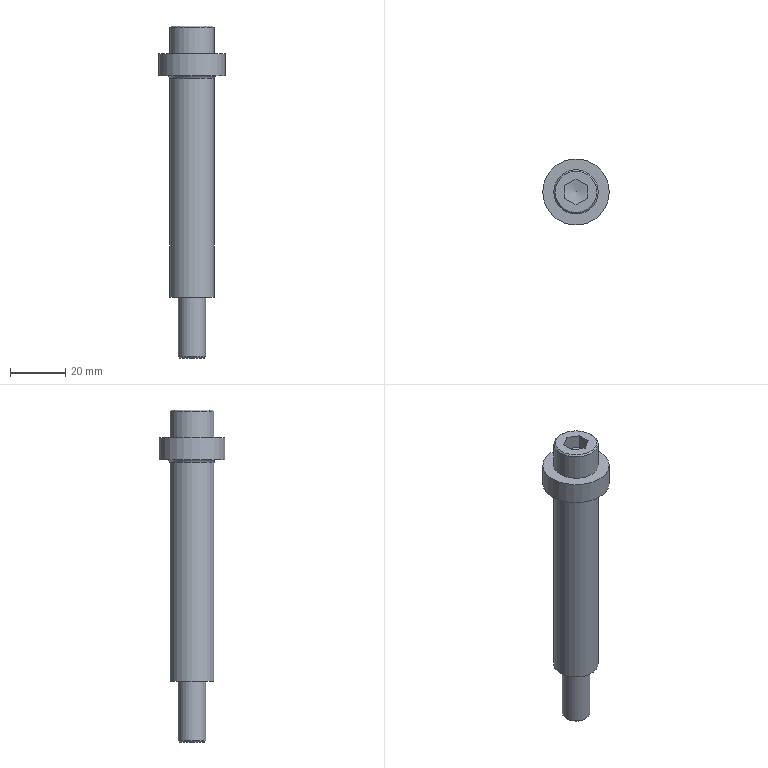Part | NX | features CSR16-70_1 2 | 1 solid | 27 faces | box 24 x 24 x 120 mm | volume 22290 mm3 | plane 18 | cylinder 5 | cone 3 | torus 1 | commonest cylinder face diameters 16 x2 10 x1 10.6 x1 24 x1
STEP:
#1=CARTESIAN_POINT('',(254.,112.,128.));
#2=VERTEX_POINT('',#1);
#3=CARTESIAN_POINT('',(266.,112.,128.));
#4=DIRECTION('',(0.,0.,-1.));
#5=DIRECTION('',(-1.,0.,0.));
#6=AXIS2_PLACEMENT_3D('',#3,#4,#5);
#7=CIRCLE('',#6,12.);
#8=EDGE_CURVE('',#2,#2,#7,.F.);
#9=ORIENTED_EDGE('',*,*,#8,.T.);
#10=EDGE_LOOP('',(#9));
#11=FACE_BOUND('',#10,.T.);
#12=CARTESIAN_POINT('',(258.,112.,128.));
#13=VERTEX_POINT('',#12);
#14=CARTESIAN_POINT('',(266.,112.,128.));
#15=DIRECTION('',(0.,0.,1.));
#16=DIRECTION('',(-1.,0.,0.));
#17=AXIS2_PLACEMENT_3D('',#14,#15,#16);
#18=CIRCLE('',#17,8.);
#19=EDGE_CURVE('',#13,#13,#18,.F.);
#20=ORIENTED_EDGE('',*,*,#19,.T.);
#21=EDGE_LOOP('',(#20));
#22=FACE_BOUND('',#21,.T.);
#23=CARTESIAN_POINT('',(266.,112.,128.));
#24=DIRECTION('',(0.,0.,1.));
#25=DIRECTION('',(-1.,0.,0.));
#26=AXIS2_PLACEMENT_3D('',#23,#24,#25);
#27=PLANE('',#26);
#28=ADVANCED_FACE('',(#11,#22),#27,.T.);
#29=CARTESIAN_POINT('',(258.,112.,119.));
#30=VERTEX_POINT('',#29);
#31=CARTESIAN_POINT('',(266.,112.,119.));
#32=DIRECTION('',(0.,0.,-1.));
#33=DIRECTION('',(1.,0.,0.));
#34=AXIS2_PLACEMENT_3D('',#31,#32,#33);
#35=CIRCLE('',#34,8.);
#36=EDGE_CURVE('',#30,#30,#35,.F.);
#37=ORIENTED_EDGE('',*,*,#36,.F.);
#38=EDGE_LOOP('',(#37));
#39=FACE_BOUND('',#38,.T.);
#40=CARTESIAN_POINT('',(258.,112.,40.));
#41=VERTEX_POINT('',#40);
#42=CARTESIAN_POINT('',(266.,112.,40.));
#43=DIRECTION('',(0.,0.,1.));
#44=DIRECTION('',(-1.,0.,0.));
#45=AXIS2_PLACEMENT_3D('',#42,#43,#44);
#46=CIRCLE('',#45,8.);
#47=EDGE_CURVE('',#41,#41,#46,.F.);
#48=ORIENTED_EDGE('',*,*,#47,.F.);
#49=EDGE_LOOP('',(#48));
#50=FACE_BOUND('',#49,.T.);
#51=CARTESIAN_POINT('',(266.,112.,75.));
#52=DIRECTION('',(0.,0.,-1.));
#53=DIRECTION('',(1.,0.,0.));
#54=AXIS2_PLACEMENT_3D('',#51,#52,#53);
#55=CYLINDRICAL_SURFACE('',#54,8.);
#56=ADVANCED_FACE('',(#39,#50),#55,.T.);
#57=CARTESIAN_POINT('',(260.7,112.,128.));
#58=VERTEX_POINT('',#57);
#59=CARTESIAN_POINT('',(266.,112.,128.));
#60=DIRECTION('',(0.,0.,1.));
#61=DIRECTION('',(-1.,0.,0.));
#62=AXIS2_PLACEMENT_3D('',#59,#60,#61);
#63=CIRCLE('',#62,5.3);
#64=EDGE_CURVE('',#58,#58,#63,.F.);
#65=ORIENTED_EDGE('',*,*,#64,.F.);
#66=EDGE_LOOP('',(#65));
#67=FACE_BOUND('',#66,.T.);
#68=CARTESIAN_POINT('',(260.7,112.,40.));
#69=VERTEX_POINT('',#68);
#70=CARTESIAN_POINT('',(266.,112.,40.));
#71=DIRECTION('',(0.,0.,-1.));
#72=DIRECTION('',(-1.,0.,0.));
#73=AXIS2_PLACEMENT_3D('',#70,#71,#72);
#74=CIRCLE('',#73,5.3);
#75=EDGE_CURVE('',#69,#69,#74,.F.);
#76=ORIENTED_EDGE('',*,*,#75,.F.);
#77=EDGE_LOOP('',(#76));
#78=FACE_BOUND('',#77,.T.);
#79=CARTESIAN_POINT('',(266.,112.,79.));
#80=DIRECTION('',(0.,0.,-1.));
#81=DIRECTION('',(1.,0.,0.));
#82=AXIS2_PLACEMENT_3D('',#79,#80,#81);
#83=CYLINDRICAL_SURFACE('',#82,5.3);
#84=ADVANCED_FACE('',(#67,#78),#83,.F.);
#85=ORIENTED_EDGE('',*,*,#36,.T.);
#86=EDGE_LOOP('',(#85));
#87=FACE_BOUND('',#86,.T.);
#88=CARTESIAN_POINT('',(257.,112.,120.));
#89=VERTEX_POINT('',#88);
#90=CARTESIAN_POINT('',(266.,112.,120.));
#91=DIRECTION('',(0.,0.,1.));
#92=DIRECTION('',(1.,0.,0.));
#93=AXIS2_PLACEMENT_3D('',#90,#91,#92);
#94=CIRCLE('',#93,9.);
#95=EDGE_CURVE('',#89,#89,#94,.F.);
#96=ORIENTED_EDGE('',*,*,#95,.T.);
#97=EDGE_LOOP('',(#96));
#98=FACE_BOUND('',#97,.T.);
#99=CARTESIAN_POINT('',(266.,112.,119.));
#100=DIRECTION('',(0.,0.,1.));
#101=DIRECTION('',(-1.,0.,0.));
#102=AXIS2_PLACEMENT_3D('',#99,#100,#101);
#103=TOROIDAL_SURFACE('',#102,9.,1.);
#104=ADVANCED_FACE('',(#87,#98),#103,.F.);
#105=CARTESIAN_POINT('',(254.,112.,120.));
#106=VERTEX_POINT('',#105);
#107=CARTESIAN_POINT('',(266.,112.,120.));
#108=DIRECTION('',(0.,0.,1.));
#109=DIRECTION('',(-1.,0.,0.));
#110=AXIS2_PLACEMENT_3D('',#107,#108,#109);
#111=CIRCLE('',#110,12.);
#112=EDGE_CURVE('',#106,#106,#111,.F.);
#113=ORIENTED_EDGE('',*,*,#112,.T.);
#114=EDGE_LOOP('',(#113));
#115=FACE_BOUND('',#114,.T.);
#116=ORIENTED_EDGE('',*,*,#95,.F.);
#117=EDGE_LOOP('',(#116));
#118=FACE_BOUND('',#117,.T.);
#119=CARTESIAN_POINT('',(266.,112.,120.));
#120=DIRECTION('',(0.,0.,-1.));
#121=DIRECTION('',(1.,0.,0.));
#122=AXIS2_PLACEMENT_3D('',#119,#120,#121);
#123=PLANE('',#122);
#124=ADVANCED_FACE('',(#115,#118),#123,.T.);
#125=ORIENTED_EDGE('',*,*,#75,.T.);
#126=EDGE_LOOP('',(#125));
#127=FACE_BOUND('',#126,.T.);
#128=ORIENTED_EDGE('',*,*,#47,.T.);
#129=EDGE_LOOP('',(#128));
#130=FACE_BOUND('',#129,.T.);
#131=CARTESIAN_POINT('',(266.,112.,40.));
#132=DIRECTION('',(0.,0.,-1.));
#133=DIRECTION('',(1.,0.,0.));
#134=AXIS2_PLACEMENT_3D('',#131,#132,#133);
#135=PLANE('',#134);
#136=ADVANCED_FACE('',(#127,#130),#135,.T.);
#137=ORIENTED_EDGE('',*,*,#8,.F.);
#138=EDGE_LOOP('',(#137));
#139=FACE_BOUND('',#138,.T.);
#140=ORIENTED_EDGE('',*,*,#112,.F.);
#141=EDGE_LOOP('',(#140));
#142=FACE_BOUND('',#141,.T.);
#143=CARTESIAN_POINT('',(266.,112.,124.));
#144=DIRECTION('',(0.,0.,-1.));
#145=DIRECTION('',(1.,0.,0.));
#146=AXIS2_PLACEMENT_3D('',#143,#144,#145);
#147=CYLINDRICAL_SURFACE('',#146,12.);
#148=ADVANCED_FACE('',(#139,#142),#147,.T.);
#149=CARTESIAN_POINT('',(262.,114.309,138.));
#150=VERTEX_POINT('',#149);
#151=CARTESIAN_POINT('',(266.,116.619,138.));
#152=VERTEX_POINT('',#151);
#153=CARTESIAN_POINT('',(264.,115.464,138.));
#154=DIRECTION('',(-0.866,-0.5,0.));
#155=VECTOR('',#154,1000.);
#156=LINE('',#153,#155);
#157=EDGE_CURVE('',#150,#152,#156,.F.);
#158=ORIENTED_EDGE('',*,*,#157,.T.);
#159=CARTESIAN_POINT('',(270.,114.309,138.));
#160=VERTEX_POINT('',#159);
#161=CARTESIAN_POINT('',(268.,115.464,138.));
#162=DIRECTION('',(-0.866,0.5,0.));
#163=VECTOR('',#162,1000.);
#164=LINE('',#161,#163);
#165=EDGE_CURVE('',#152,#160,#164,.F.);
#166=ORIENTED_EDGE('',*,*,#165,.T.);
#167=CARTESIAN_POINT('',(270.,109.691,138.));
#168=VERTEX_POINT('',#167);
#169=CARTESIAN_POINT('',(270.,112.,138.));
#170=DIRECTION('',(0.,1.,0.));
#171=VECTOR('',#170,1000.);
#172=LINE('',#169,#171);
#173=EDGE_CURVE('',#160,#168,#172,.F.);
#174=ORIENTED_EDGE('',*,*,#173,.T.);
#175=CARTESIAN_POINT('',(266.,107.381,138.));
#176=VERTEX_POINT('',#175);
#177=CARTESIAN_POINT('',(268.,108.536,138.));
#178=DIRECTION('',(0.866,0.5,0.));
#179=VECTOR('',#178,1000.);
#180=LINE('',#177,#179);
#181=EDGE_CURVE('',#168,#176,#180,.F.);
#182=ORIENTED_EDGE('',*,*,#181,.T.);
#183=CARTESIAN_POINT('',(262.,109.691,138.));
#184=VERTEX_POINT('',#183);
#185=CARTESIAN_POINT('',(264.,108.536,138.));
#186=DIRECTION('',(0.866,-0.5,0.));
#187=VECTOR('',#186,1000.);
#188=LINE('',#185,#187);
#189=EDGE_CURVE('',#176,#184,#188,.F.);
#190=ORIENTED_EDGE('',*,*,#189,.T.);
#191=CARTESIAN_POINT('',(262.,112.,138.));
#192=DIRECTION('',(0.,-1.,0.));
#193=VECTOR('',#192,1000.);
#194=LINE('',#191,#193);
#195=EDGE_CURVE('',#184,#150,#194,.F.);
#196=ORIENTED_EDGE('',*,*,#195,.T.);
#197=EDGE_LOOP('',(#158,#166,#174,#182,#190,#196));
#198=FACE_BOUND('',#197,.T.);
#199=CARTESIAN_POINT('',(258.5,112.,138.));
#200=VERTEX_POINT('',#199);
#201=CARTESIAN_POINT('',(266.,112.,138.));
#202=DIRECTION('',(0.,0.,1.));
#203=DIRECTION('',(1.,0.,0.));
#204=AXIS2_PLACEMENT_3D('',#201,#202,#203);
#205=CIRCLE('',#204,7.5);
#206=EDGE_CURVE('',#200,#200,#205,.F.);
#207=ORIENTED_EDGE('',*,*,#206,.F.);
#208=EDGE_LOOP('',(#207));
#209=FACE_BOUND('',#208,.T.);
#210=CARTESIAN_POINT('',(266.,112.,138.));
#211=DIRECTION('',(0.,0.,1.));
#212=DIRECTION('',(-1.,0.,0.));
#213=AXIS2_PLACEMENT_3D('',#210,#211,#212);
#214=PLANE('',#213);
#215=ADVANCED_FACE('',(#198,#209),#214,.T.);
#216=ORIENTED_EDGE('',*,*,#19,.F.);
#217=EDGE_LOOP('',(#216));
#218=FACE_BOUND('',#217,.T.);
#219=CARTESIAN_POINT('',(258.,112.,137.5));
#220=VERTEX_POINT('',#219);
#221=CARTESIAN_POINT('',(266.,112.,137.5));
#222=DIRECTION('',(0.,0.,-1.));
#223=DIRECTION('',(1.,0.,0.));
#224=AXIS2_PLACEMENT_3D('',#221,#222,#223);
#225=CIRCLE('',#224,8.);
#226=EDGE_CURVE('',#220,#220,#225,.F.);
#227=ORIENTED_EDGE('',*,*,#226,.F.);
#228=EDGE_LOOP('',(#227));
#229=FACE_BOUND('',#228,.T.);
#230=CARTESIAN_POINT('',(266.,112.,133.));
#231=DIRECTION('',(0.,0.,-1.));
#232=DIRECTION('',(1.,0.,0.));
#233=AXIS2_PLACEMENT_3D('',#230,#231,#232);
#234=CYLINDRICAL_SURFACE('',#233,8.);
#235=ADVANCED_FACE('',(#218,#229),#234,.T.);
#236=ORIENTED_EDGE('',*,*,#226,.T.);
#237=EDGE_LOOP('',(#236));
#238=FACE_BOUND('',#237,.T.);
#239=ORIENTED_EDGE('',*,*,#206,.T.);
#240=EDGE_LOOP('',(#239));
#241=FACE_BOUND('',#240,.T.);
#242=CARTESIAN_POINT('',(266.,112.,138.));
#243=DIRECTION('',(0.,0.,-1.));
#244=DIRECTION('',(-1.,0.,0.));
#245=AXIS2_PLACEMENT_3D('',#242,#243,#244);
#246=CONICAL_SURFACE('',#245,7.5,0.7854);
#247=ADVANCED_FACE('',(#238,#241),#246,.T.);
#248=CARTESIAN_POINT('',(262.,114.309,133.));
#249=VERTEX_POINT('',#248);
#250=CARTESIAN_POINT('',(262.,114.309,135.5));
#251=DIRECTION('',(0.,0.,1.));
#252=VECTOR('',#251,1000.);
#253=LINE('',#250,#252);
#254=EDGE_CURVE('',#150,#249,#253,.F.);
#255=ORIENTED_EDGE('',*,*,#254,.F.);
#256=ORIENTED_EDGE('',*,*,#195,.F.);
#257=CARTESIAN_POINT('',(262.,109.691,133.));
#258=VERTEX_POINT('',#257);
#259=CARTESIAN_POINT('',(262.,109.691,135.5));
#260=DIRECTION('',(0.,0.,1.));
#261=VECTOR('',#260,1000.);
#262=LINE('',#259,#261);
#263=EDGE_CURVE('',#184,#258,#262,.F.);
#264=ORIENTED_EDGE('',*,*,#263,.T.);
#265=CARTESIAN_POINT('',(262.,112.,133.));
#266=DIRECTION('',(0.,-1.,0.));
#267=VECTOR('',#266,1000.);
#268=LINE('',#265,#267);
#269=EDGE_CURVE('',#258,#249,#268,.F.);
#270=ORIENTED_EDGE('',*,*,#269,.T.);
#271=EDGE_LOOP('',(#255,#256,#264,#270));
#272=FACE_BOUND('',#271,.T.);
#273=CARTESIAN_POINT('',(262.,112.,135.5));
#274=DIRECTION('',(1.,0.,0.));
#275=DIRECTION('',(0.,0.,1.));
#276=AXIS2_PLACEMENT_3D('',#273,#274,#275);
#277=PLANE('',#276);
#278=ADVANCED_FACE('',(#272),#277,.T.);
#279=ORIENTED_EDGE('',*,*,#263,.F.);
#280=ORIENTED_EDGE('',*,*,#189,.F.);
#281=CARTESIAN_POINT('',(266.,107.381,133.));
#282=VERTEX_POINT('',#281);
#283=CARTESIAN_POINT('',(266.,107.381,135.5));
#284=DIRECTION('',(0.,0.,1.));
#285=VECTOR('',#284,1000.);
#286=LINE('',#283,#285);
#287=EDGE_CURVE('',#176,#282,#286,.F.);
#288=ORIENTED_EDGE('',*,*,#287,.T.);
#289=CARTESIAN_POINT('',(264.,108.536,133.));
#290=DIRECTION('',(0.866,-0.5,0.));
#291=VECTOR('',#290,1000.);
#292=LINE('',#289,#291);
#293=EDGE_CURVE('',#282,#258,#292,.F.);
#294=ORIENTED_EDGE('',*,*,#293,.T.);
#295=EDGE_LOOP('',(#279,#280,#288,#294));
#296=FACE_BOUND('',#295,.T.);
#297=CARTESIAN_POINT('',(264.,108.536,135.5));
#298=DIRECTION('',(0.5,0.866,0.));
#299=DIRECTION('',(0.,0.,1.));
#300=AXIS2_PLACEMENT_3D('',#297,#298,#299);
#301=PLANE('',#300);
#302=ADVANCED_FACE('',(#296),#301,.T.);
#303=ORIENTED_EDGE('',*,*,#287,.F.);
#304=ORIENTED_EDGE('',*,*,#181,.F.);
#305=CARTESIAN_POINT('',(270.,109.691,133.));
#306=VERTEX_POINT('',#305);
#307=CARTESIAN_POINT('',(270.,109.691,135.5));
#308=DIRECTION('',(0.,0.,1.));
#309=VECTOR('',#308,1000.);
#310=LINE('',#307,#309);
#311=EDGE_CURVE('',#168,#306,#310,.F.);
#312=ORIENTED_EDGE('',*,*,#311,.T.);
#313=CARTESIAN_POINT('',(268.,108.536,133.));
#314=DIRECTION('',(0.866,0.5,0.));
#315=VECTOR('',#314,1000.);
#316=LINE('',#313,#315);
#317=EDGE_CURVE('',#306,#282,#316,.F.);
#318=ORIENTED_EDGE('',*,*,#317,.T.);
#319=EDGE_LOOP('',(#303,#304,#312,#318));
#320=FACE_BOUND('',#319,.T.);
#321=CARTESIAN_POINT('',(268.,108.536,135.5));
#322=DIRECTION('',(-0.5,0.866,0.));
#323=DIRECTION('',(0.,0.,-1.));
#324=AXIS2_PLACEMENT_3D('',#321,#322,#323);
#325=PLANE('',#324);
#326=ADVANCED_FACE('',(#320),#325,.T.);
#327=ORIENTED_EDGE('',*,*,#311,.F.);
#328=ORIENTED_EDGE('',*,*,#173,.F.);
#329=CARTESIAN_POINT('',(270.,114.309,133.));
#330=VERTEX_POINT('',#329);
#331=CARTESIAN_POINT('',(270.,114.309,135.5));
#332=DIRECTION('',(0.,0.,1.));
#333=VECTOR('',#332,1000.);
#334=LINE('',#331,#333);
#335=EDGE_CURVE('',#160,#330,#334,.F.);
#336=ORIENTED_EDGE('',*,*,#335,.T.);
#337=CARTESIAN_POINT('',(270.,112.,133.));
#338=DIRECTION('',(0.,1.,0.));
#339=VECTOR('',#338,1000.);
#340=LINE('',#337,#339);
#341=EDGE_CURVE('',#330,#306,#340,.F.);
#342=ORIENTED_EDGE('',*,*,#341,.T.);
#343=EDGE_LOOP('',(#327,#328,#336,#342));
#344=FACE_BOUND('',#343,.T.);
#345=CARTESIAN_POINT('',(270.,112.,135.5));
#346=DIRECTION('',(-1.,0.,0.));
#347=DIRECTION('',(0.,0.,-1.));
#348=AXIS2_PLACEMENT_3D('',#345,#346,#347);
#349=PLANE('',#348);
#350=ADVANCED_FACE('',(#344),#349,.T.);
#351=ORIENTED_EDGE('',*,*,#335,.F.);
#352=ORIENTED_EDGE('',*,*,#165,.F.);
#353=CARTESIAN_POINT('',(266.,116.619,133.));
#354=VERTEX_POINT('',#353);
#355=CARTESIAN_POINT('',(266.,116.619,135.5));
#356=DIRECTION('',(0.,0.,1.));
#357=VECTOR('',#356,1000.);
#358=LINE('',#355,#357);
#359=EDGE_CURVE('',#152,#354,#358,.F.);
#360=ORIENTED_EDGE('',*,*,#359,.T.);
#361=CARTESIAN_POINT('',(268.,115.464,133.));
#362=DIRECTION('',(-0.866,0.5,0.));
#363=VECTOR('',#362,1000.);
#364=LINE('',#361,#363);
#365=EDGE_CURVE('',#354,#330,#364,.F.);
#366=ORIENTED_EDGE('',*,*,#365,.T.);
#367=EDGE_LOOP('',(#351,#352,#360,#366));
#368=FACE_BOUND('',#367,.T.);
#369=CARTESIAN_POINT('',(268.,115.464,135.5));
#370=DIRECTION('',(-0.5,-0.866,0.));
#371=DIRECTION('',(0.,0.,-1.));
#372=AXIS2_PLACEMENT_3D('',#369,#370,#371);
#373=PLANE('',#372);
#374=ADVANCED_FACE('',(#368),#373,.T.);
#375=ORIENTED_EDGE('',*,*,#359,.F.);
#376=ORIENTED_EDGE('',*,*,#157,.F.);
#377=ORIENTED_EDGE('',*,*,#254,.T.);
#378=CARTESIAN_POINT('',(264.,115.464,133.));
#379=DIRECTION('',(-0.866,-0.5,0.));
#380=VECTOR('',#379,1000.);
#381=LINE('',#378,#380);
#382=EDGE_CURVE('',#249,#354,#381,.F.);
#383=ORIENTED_EDGE('',*,*,#382,.T.);
#384=EDGE_LOOP('',(#375,#376,#377,#383));
#385=FACE_BOUND('',#384,.T.);
#386=CARTESIAN_POINT('',(264.,115.464,135.5));
#387=DIRECTION('',(0.5,-0.866,0.));
#388=DIRECTION('',(0.,0.,1.));
#389=AXIS2_PLACEMENT_3D('',#386,#387,#388);
#390=PLANE('',#389);
#391=ADVANCED_FACE('',(#385),#390,.T.);
#392=CARTESIAN_POINT('',(266.,112.,133.));
#393=DIRECTION('',(0.,0.,-1.));
#394=DIRECTION('',(-1.,0.,0.));
#395=AXIS2_PLACEMENT_3D('',#392,#393,#394);
#396=CIRCLE('',#395,4.619);
#397=EDGE_CURVE('',#249,#258,#396,.F.);
#398=ORIENTED_EDGE('',*,*,#397,.T.);
#399=CARTESIAN_POINT('',(266.,112.,133.));
#400=DIRECTION('',(0.,0.,-1.));
#401=DIRECTION('',(-1.,0.,0.));
#402=AXIS2_PLACEMENT_3D('',#399,#400,#401);
#403=CIRCLE('',#402,4.619);
#404=EDGE_CURVE('',#258,#282,#403,.F.);
#405=ORIENTED_EDGE('',*,*,#404,.T.);
#406=CARTESIAN_POINT('',(266.,112.,133.));
#407=DIRECTION('',(0.,0.,-1.));
#408=DIRECTION('',(-1.,0.,0.));
#409=AXIS2_PLACEMENT_3D('',#406,#407,#408);
#410=CIRCLE('',#409,4.619);
#411=EDGE_CURVE('',#282,#306,#410,.F.);
#412=ORIENTED_EDGE('',*,*,#411,.T.);
#413=CARTESIAN_POINT('',(266.,112.,133.));
#414=DIRECTION('',(0.,0.,-1.));
#415=DIRECTION('',(-1.,0.,0.));
#416=AXIS2_PLACEMENT_3D('',#413,#414,#415);
#417=CIRCLE('',#416,4.619);
#418=EDGE_CURVE('',#306,#330,#417,.F.);
#419=ORIENTED_EDGE('',*,*,#418,.T.);
#420=CARTESIAN_POINT('',(266.,112.,133.));
#421=DIRECTION('',(0.,0.,-1.));
#422=DIRECTION('',(-1.,0.,0.));
#423=AXIS2_PLACEMENT_3D('',#420,#421,#422);
#424=CIRCLE('',#423,4.619);
#425=EDGE_CURVE('',#330,#354,#424,.F.);
#426=ORIENTED_EDGE('',*,*,#425,.T.);
#427=CARTESIAN_POINT('',(266.,112.,133.));
#428=DIRECTION('',(0.,0.,-1.));
#429=DIRECTION('',(-1.,0.,0.));
#430=AXIS2_PLACEMENT_3D('',#427,#428,#429);
#431=CIRCLE('',#430,4.619);
#432=EDGE_CURVE('',#354,#249,#431,.F.);
#433=ORIENTED_EDGE('',*,*,#432,.T.);
#434=EDGE_LOOP('',(#398,#405,#412,#419,#426,#433));
#435=FACE_BOUND('',#434,.T.);
#436=CARTESIAN_POINT('',(266.,112.,132.));
#437=VERTEX_POINT('',#436);
#438=VERTEX_LOOP('',#437);
#439=FACE_BOUND('',#438,.T.);
#440=CARTESIAN_POINT('',(266.,112.,132.5));
#441=DIRECTION('',(0.,0.,1.));
#442=DIRECTION('',(1.,0.,0.));
#443=AXIS2_PLACEMENT_3D('',#440,#441,#442);
#444=CONICAL_SURFACE('',#443,2.309,1.358);
#445=ADVANCED_FACE('',(#435,#439),#444,.F.);
#446=ORIENTED_EDGE('',*,*,#365,.F.);
#447=ORIENTED_EDGE('',*,*,#425,.F.);
#448=EDGE_LOOP('',(#446,#447));
#449=FACE_BOUND('',#448,.T.);
#450=CARTESIAN_POINT('',(266.,112.,133.));
#451=DIRECTION('',(0.,0.,1.));
#452=DIRECTION('',(-1.,0.,0.));
#453=AXIS2_PLACEMENT_3D('',#450,#451,#452);
#454=PLANE('',#453);
#455=ADVANCED_FACE('',(#449),#454,.F.);
#456=ORIENTED_EDGE('',*,*,#341,.F.);
#457=ORIENTED_EDGE('',*,*,#418,.F.);
#458=EDGE_LOOP('',(#456,#457));
#459=FACE_BOUND('',#458,.T.);
#460=CARTESIAN_POINT('',(266.,112.,133.));
#461=DIRECTION('',(0.,0.,1.));
#462=DIRECTION('',(-1.,0.,0.));
#463=AXIS2_PLACEMENT_3D('',#460,#461,#462);
#464=PLANE('',#463);
#465=ADVANCED_FACE('',(#459),#464,.F.);
#466=ORIENTED_EDGE('',*,*,#317,.F.);
#467=ORIENTED_EDGE('',*,*,#411,.F.);
#468=EDGE_LOOP('',(#466,#467));
#469=FACE_BOUND('',#468,.T.);
#470=CARTESIAN_POINT('',(266.,112.,133.));
#471=DIRECTION('',(0.,0.,1.));
#472=DIRECTION('',(-1.,0.,0.));
#473=AXIS2_PLACEMENT_3D('',#470,#471,#472);
#474=PLANE('',#473);
#475=ADVANCED_FACE('',(#469),#474,.F.);
#476=ORIENTED_EDGE('',*,*,#293,.F.);
#477=ORIENTED_EDGE('',*,*,#404,.F.);
#478=EDGE_LOOP('',(#476,#477));
#479=FACE_BOUND('',#478,.T.);
#480=CARTESIAN_POINT('',(266.,112.,133.));
#481=DIRECTION('',(0.,0.,1.));
#482=DIRECTION('',(-1.,0.,0.));
#483=AXIS2_PLACEMENT_3D('',#480,#481,#482);
#484=PLANE('',#483);
#485=ADVANCED_FACE('',(#479),#484,.F.);
#486=ORIENTED_EDGE('',*,*,#269,.F.);
#487=ORIENTED_EDGE('',*,*,#397,.F.);
#488=EDGE_LOOP('',(#486,#487));
#489=FACE_BOUND('',#488,.T.);
#490=CARTESIAN_POINT('',(266.,112.,133.));
#491=DIRECTION('',(0.,0.,1.));
#492=DIRECTION('',(-1.,0.,0.));
#493=AXIS2_PLACEMENT_3D('',#490,#491,#492);
#494=PLANE('',#493);
#495=ADVANCED_FACE('',(#489),#494,.F.);
#496=ORIENTED_EDGE('',*,*,#382,.F.);
#497=ORIENTED_EDGE('',*,*,#432,.F.);
#498=EDGE_LOOP('',(#496,#497));
#499=FACE_BOUND('',#498,.T.);
#500=CARTESIAN_POINT('',(266.,112.,133.));
#501=DIRECTION('',(0.,0.,1.));
#502=DIRECTION('',(-1.,0.,0.));
#503=AXIS2_PLACEMENT_3D('',#500,#501,#502);
#504=PLANE('',#503);
#505=ADVANCED_FACE('',(#499),#504,.F.);
#506=CARTESIAN_POINT('',(261.,112.,18.5));
#507=VERTEX_POINT('',#506);
#508=CARTESIAN_POINT('',(266.,112.,18.5));
#509=DIRECTION('',(0.,0.,1.));
#510=DIRECTION('',(1.,0.,0.));
#511=AXIS2_PLACEMENT_3D('',#508,#509,#510);
#512=CIRCLE('',#511,5.);
#513=EDGE_CURVE('',#507,#507,#512,.F.);
#514=ORIENTED_EDGE('',*,*,#513,.T.);
#515=EDGE_LOOP('',(#514));
#516=FACE_BOUND('',#515,.T.);
#517=CARTESIAN_POINT('',(261.5,112.,18.));
#518=VERTEX_POINT('',#517);
#519=CARTESIAN_POINT('',(266.,112.,18.));
#520=DIRECTION('',(0.,0.,-1.));
#521=DIRECTION('',(1.,0.,0.));
#522=AXIS2_PLACEMENT_3D('',#519,#520,#521);
#523=CIRCLE('',#522,4.5);
#524=EDGE_CURVE('',#518,#518,#523,.F.);
#525=ORIENTED_EDGE('',*,*,#524,.T.);
#526=EDGE_LOOP('',(#525));
#527=FACE_BOUND('',#526,.T.);
#528=CARTESIAN_POINT('',(266.,112.,18.));
#529=DIRECTION('',(0.,0.,1.));
#530=DIRECTION('',(-1.,0.,0.));
#531=AXIS2_PLACEMENT_3D('',#528,#529,#530);
#532=CONICAL_SURFACE('',#531,4.5,0.7854);
#533=ADVANCED_FACE('',(#516,#527),#532,.T.);
#534=CARTESIAN_POINT('',(261.,112.,128.));
#535=VERTEX_POINT('',#534);
#536=CARTESIAN_POINT('',(266.,112.,128.));
#537=DIRECTION('',(0.,0.,-1.));
#538=DIRECTION('',(-1.,0.,0.));
#539=AXIS2_PLACEMENT_3D('',#536,#537,#538);
#540=CIRCLE('',#539,5.);
#541=EDGE_CURVE('',#535,#535,#540,.F.);
#542=ORIENTED_EDGE('',*,*,#541,.F.);
#543=EDGE_LOOP('',(#542));
#544=FACE_BOUND('',#543,.T.);
#545=ORIENTED_EDGE('',*,*,#513,.F.);
#546=EDGE_LOOP('',(#545));
#547=FACE_BOUND('',#546,.T.);
#548=CARTESIAN_POINT('',(266.,112.,68.));
#549=DIRECTION('',(0.,0.,-1.));
#550=DIRECTION('',(1.,0.,0.));
#551=AXIS2_PLACEMENT_3D('',#548,#549,#550);
#552=CYLINDRICAL_SURFACE('',#551,5.);
#553=ADVANCED_FACE('',(#544,#547),#552,.T.);
#554=ORIENTED_EDGE('',*,*,#524,.F.);
#555=EDGE_LOOP('',(#554));
#556=FACE_BOUND('',#555,.T.);
#557=CARTESIAN_POINT('',(266.,112.,18.));
#558=DIRECTION('',(0.,0.,-1.));
#559=DIRECTION('',(1.,0.,0.));
#560=AXIS2_PLACEMENT_3D('',#557,#558,#559);
#561=PLANE('',#560);
#562=ADVANCED_FACE('',(#556),#561,.T.);
#563=ORIENTED_EDGE('',*,*,#64,.T.);
#564=EDGE_LOOP('',(#563));
#565=FACE_BOUND('',#564,.T.);
#566=ORIENTED_EDGE('',*,*,#541,.T.);
#567=EDGE_LOOP('',(#566));
#568=FACE_BOUND('',#567,.T.);
#569=CARTESIAN_POINT('',(266.,112.,128.));
#570=DIRECTION('',(0.,0.,-1.));
#571=DIRECTION('',(1.,0.,0.));
#572=AXIS2_PLACEMENT_3D('',#569,#570,#571);
#573=PLANE('',#572);
#574=ADVANCED_FACE('',(#565,#568),#573,.T.);
#575=CLOSED_SHELL('',(#28,#56,#84,#104,#124,#136,#148,#215,#235,#247,#278,#302,#326,#350,#374,#391,#445,#455,#465,#475,#485,#495,#505,#533,#553,#562,#574));
#576=MANIFOLD_SOLID_BREP('',#575);
#577=(LENGTH_UNIT()NAMED_UNIT(*)SI_UNIT(.MILLI.,.METRE.));
#578=UNCERTAINTY_MEASURE_WITH_UNIT(LENGTH_MEASURE(0.00001),#577,'','');
#579=(NAMED_UNIT(*)PLANE_ANGLE_UNIT()SI_UNIT($,.RADIAN.));
#580=(NAMED_UNIT(*)SI_UNIT($,.STERADIAN.)SOLID_ANGLE_UNIT());
#581=(GEOMETRIC_REPRESENTATION_CONTEXT(3)GLOBAL_UNCERTAINTY_ASSIGNED_CONTEXT((#578))GLOBAL_UNIT_ASSIGNED_CONTEXT((#577,#579,#580))REPRESENTATION_CONTEXT('',''));
#582=ADVANCED_BREP_SHAPE_REPRESENTATION('',(#576),#581);